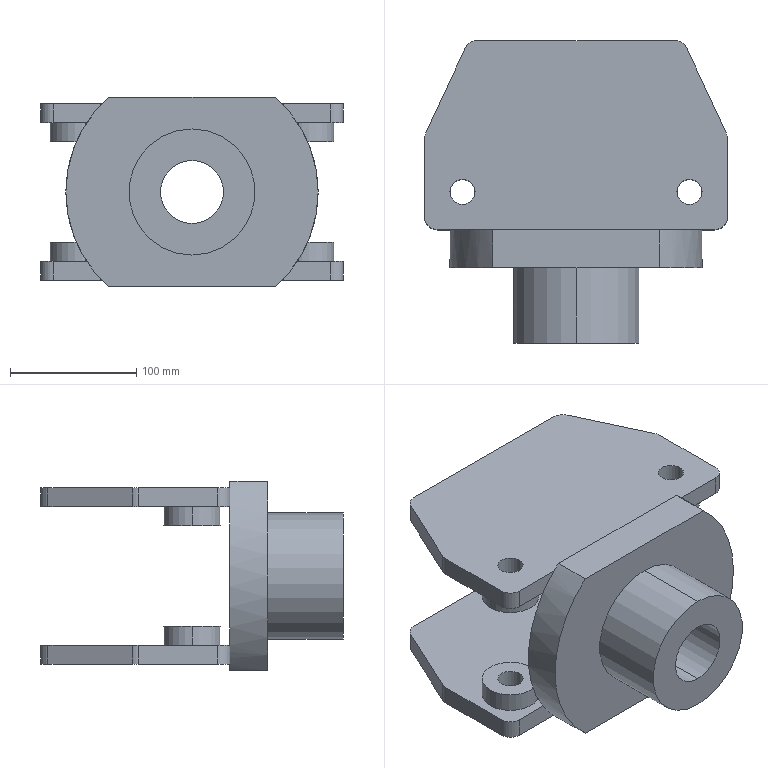Part | SolidWorks | features ICE 9, Fillet 2, Extrusion 1 | 5 solids | 75 faces | box 240 x 240 x 150 mm | volume 2158258 mm3 | cylinder 42 | plane 33 | commonest cylinder face diameters 20 x28 45 x8 50 x2 100 x2 200 x2